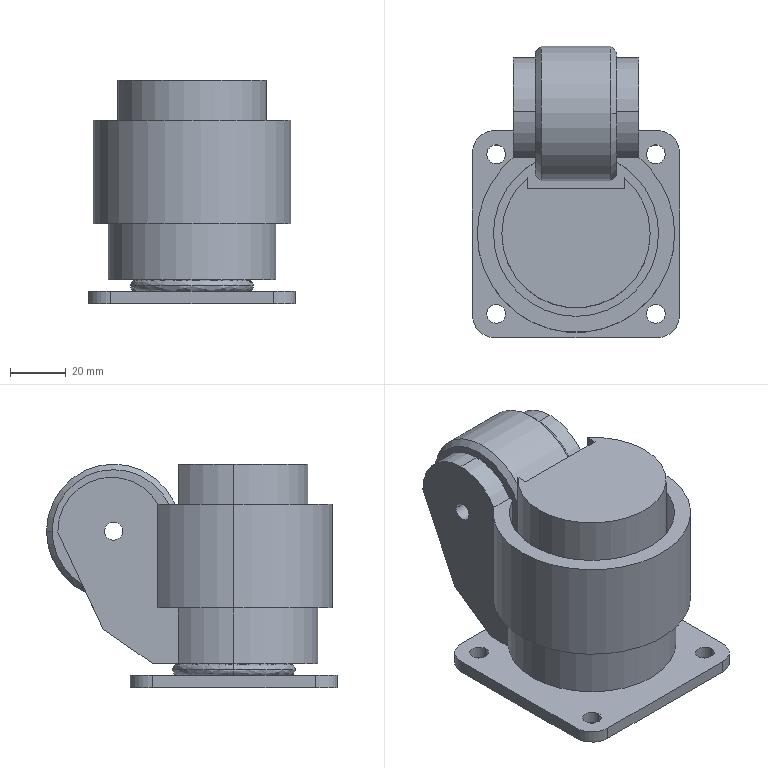Part | STEP file | FM wheel (3 inch) | 3 solids | 67 faces | box 74 x 103.967 x 80 mm | volume 304180 mm3 | cylinder 32 | plane 26 | cone 5 | spline 4 | commonest cylinder face diameters 6.7 x8 16 x4 38.335 x4 53 x3 59 x3 60 x3